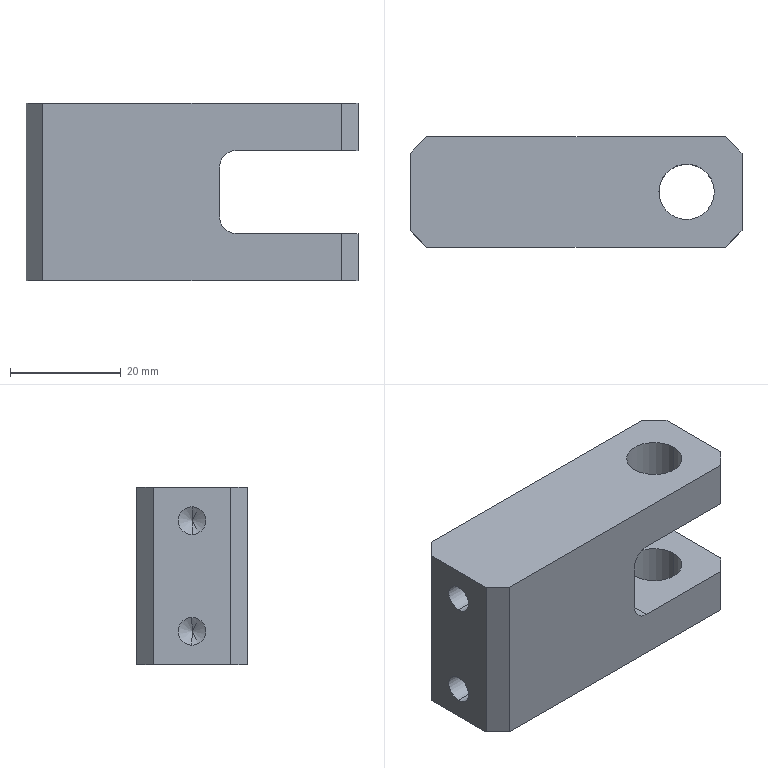Part | SolidWorks | features ICE 2, Chamfer 1, Extrusion 1, Fillet 1, HoleWzd 1 | 1 solid | 30 faces | box 60 x 20 x 32 mm | volume 28592 mm3 | plane 16 | cylinder 10 | cone 4 | commonest cylinder face diameters 5 x4 10 x4 6 x2
STEP:
#1=CARTESIAN_POINT('',(-15.,10.,-12.5));
#2=VERTEX_POINT('',#1);
#3=CARTESIAN_POINT('',(-15.,10.,-7.5));
#4=VERTEX_POINT('',#3);
#5=CARTESIAN_POINT('',(-15.,10.,-10.));
#6=DIRECTION('',(-1.,0.,0.));
#7=DIRECTION('',(0.,0.,1.));
#8=AXIS2_PLACEMENT_3D('',#5,#6,#7);
#9=CIRCLE('',#8,2.5);
#10=EDGE_CURVE('',#2,#4,#9,.T.);
#11=ORIENTED_EDGE('',*,*,#10,.F.);
#12=CARTESIAN_POINT('',(-30.,10.,-12.5));
#13=VERTEX_POINT('',#12);
#14=CARTESIAN_POINT('',(-30.,10.,-12.5));
#15=DIRECTION('',(-1.,0.,0.));
#16=VECTOR('',#15,1000.);
#17=LINE('',#14,#16);
#18=EDGE_CURVE('',#2,#13,#17,.T.);
#19=ORIENTED_EDGE('',*,*,#18,.T.);
#20=CARTESIAN_POINT('',(-30.,10.,-7.5));
#21=VERTEX_POINT('',#20);
#22=CARTESIAN_POINT('',(-30.,10.,-10.));
#23=DIRECTION('',(-1.,0.,0.));
#24=DIRECTION('',(0.,0.,1.));
#25=AXIS2_PLACEMENT_3D('',#22,#23,#24);
#26=CIRCLE('',#25,2.5);
#27=EDGE_CURVE('',#13,#21,#26,.T.);
#28=ORIENTED_EDGE('',*,*,#27,.T.);
#29=CARTESIAN_POINT('',(-30.,10.,-7.5));
#30=DIRECTION('',(-1.,0.,0.));
#31=VECTOR('',#30,1000.);
#32=LINE('',#29,#31);
#33=EDGE_CURVE('',#4,#21,#32,.T.);
#34=ORIENTED_EDGE('',*,*,#33,.F.);
#35=EDGE_LOOP('',(#11,#19,#28,#34));
#36=FACE_OUTER_BOUND('',#35,.T.);
#37=CARTESIAN_POINT('',(-30.,10.,-10.));
#38=DIRECTION('',(-1.,0.,0.));
#39=DIRECTION('',(0.,0.,1.));
#40=AXIS2_PLACEMENT_3D('',#37,#38,#39);
#41=CYLINDRICAL_SURFACE('',#40,2.5);
#42=ADVANCED_FACE('',(#36),#41,.F.);
#43=CARTESIAN_POINT('',(-13.498,10.,-10.));
#44=VERTEX_POINT('',#43);
#45=CARTESIAN_POINT('',(-15.,10.,-7.5));
#46=DIRECTION('',(-0.515,0.,0.8572));
#47=VECTOR('',#46,1000.);
#48=LINE('',#45,#47);
#49=EDGE_CURVE('',#44,#4,#48,.T.);
#50=ORIENTED_EDGE('',*,*,#49,.F.);
#51=CARTESIAN_POINT('',(-15.,10.,-12.5));
#52=DIRECTION('',(-0.515,0.,-0.8572));
#53=VECTOR('',#52,1000.);
#54=LINE('',#51,#53);
#55=EDGE_CURVE('',#44,#2,#54,.T.);
#56=ORIENTED_EDGE('',*,*,#55,.T.);
#57=ORIENTED_EDGE('',*,*,#10,.T.);
#58=EDGE_LOOP('',(#50,#56,#57));
#59=FACE_OUTER_BOUND('',#58,.T.);
#60=CARTESIAN_POINT('',(-15.,10.,-10.));
#61=DIRECTION('',(-1.,0.,0.));
#62=DIRECTION('',(0.,0.,1.));
#63=AXIS2_PLACEMENT_3D('',#60,#61,#62);
#64=CONICAL_SURFACE('',#63,2.5,1.03);
#65=ADVANCED_FACE('',(#59),#64,.F.);
#66=CARTESIAN_POINT('',(-15.,10.,7.5));
#67=VERTEX_POINT('',#66);
#68=CARTESIAN_POINT('',(-15.,10.,12.5));
#69=VERTEX_POINT('',#68);
#70=CARTESIAN_POINT('',(-15.,10.,10.));
#71=DIRECTION('',(-1.,0.,0.));
#72=DIRECTION('',(0.,0.,1.));
#73=AXIS2_PLACEMENT_3D('',#70,#71,#72);
#74=CIRCLE('',#73,2.5);
#75=EDGE_CURVE('',#67,#69,#74,.T.);
#76=ORIENTED_EDGE('',*,*,#75,.F.);
#77=CARTESIAN_POINT('',(-30.,10.,7.5));
#78=VERTEX_POINT('',#77);
#79=CARTESIAN_POINT('',(-30.,10.,7.5));
#80=DIRECTION('',(-1.,0.,0.));
#81=VECTOR('',#80,1000.);
#82=LINE('',#79,#81);
#83=EDGE_CURVE('',#67,#78,#82,.T.);
#84=ORIENTED_EDGE('',*,*,#83,.T.);
#85=CARTESIAN_POINT('',(-30.,10.,12.5));
#86=VERTEX_POINT('',#85);
#87=CARTESIAN_POINT('',(-30.,10.,10.));
#88=DIRECTION('',(-1.,0.,0.));
#89=DIRECTION('',(0.,0.,1.));
#90=AXIS2_PLACEMENT_3D('',#87,#88,#89);
#91=CIRCLE('',#90,2.5);
#92=EDGE_CURVE('',#78,#86,#91,.T.);
#93=ORIENTED_EDGE('',*,*,#92,.T.);
#94=CARTESIAN_POINT('',(-30.,10.,12.5));
#95=DIRECTION('',(-1.,0.,0.));
#96=VECTOR('',#95,1000.);
#97=LINE('',#94,#96);
#98=EDGE_CURVE('',#69,#86,#97,.T.);
#99=ORIENTED_EDGE('',*,*,#98,.F.);
#100=EDGE_LOOP('',(#76,#84,#93,#99));
#101=FACE_OUTER_BOUND('',#100,.T.);
#102=CARTESIAN_POINT('',(-30.,10.,10.));
#103=DIRECTION('',(-1.,0.,0.));
#104=DIRECTION('',(0.,0.,1.));
#105=AXIS2_PLACEMENT_3D('',#102,#103,#104);
#106=CYLINDRICAL_SURFACE('',#105,2.5);
#107=ADVANCED_FACE('',(#101),#106,.F.);
#108=CARTESIAN_POINT('',(-13.498,10.,10.));
#109=VERTEX_POINT('',#108);
#110=CARTESIAN_POINT('',(-15.,10.,12.5));
#111=DIRECTION('',(-0.515,0.,0.8572));
#112=VECTOR('',#111,1000.);
#113=LINE('',#110,#112);
#114=EDGE_CURVE('',#109,#69,#113,.T.);
#115=ORIENTED_EDGE('',*,*,#114,.F.);
#116=CARTESIAN_POINT('',(-15.,10.,7.5));
#117=DIRECTION('',(-0.515,0.,-0.8572));
#118=VECTOR('',#117,1000.);
#119=LINE('',#116,#118);
#120=EDGE_CURVE('',#109,#67,#119,.T.);
#121=ORIENTED_EDGE('',*,*,#120,.T.);
#122=ORIENTED_EDGE('',*,*,#75,.T.);
#123=EDGE_LOOP('',(#115,#121,#122));
#124=FACE_OUTER_BOUND('',#123,.T.);
#125=CARTESIAN_POINT('',(-15.,10.,10.));
#126=DIRECTION('',(-1.,0.,0.));
#127=DIRECTION('',(0.,0.,1.));
#128=AXIS2_PLACEMENT_3D('',#125,#126,#127);
#129=CONICAL_SURFACE('',#128,2.5,1.03);
#130=ADVANCED_FACE('',(#124),#129,.F.);
#131=CARTESIAN_POINT('',(25.,10.,7.5));
#132=VERTEX_POINT('',#131);
#133=CARTESIAN_POINT('',(15.,10.,7.5));
#134=VERTEX_POINT('',#133);
#135=CARTESIAN_POINT('',(20.,10.,7.5));
#136=DIRECTION('',(0.,0.,-1.));
#137=DIRECTION('',(1.,0.,0.));
#138=AXIS2_PLACEMENT_3D('',#135,#136,#137);
#139=CIRCLE('',#138,5.);
#140=EDGE_CURVE('',#132,#134,#139,.T.);
#141=ORIENTED_EDGE('',*,*,#140,.T.);
#142=CARTESIAN_POINT('',(15.,10.,16.));
#143=VERTEX_POINT('',#142);
#144=CARTESIAN_POINT('',(15.,10.,-26.));
#145=DIRECTION('',(0.,0.,1.));
#146=VECTOR('',#145,1000.);
#147=LINE('',#144,#146);
#148=EDGE_CURVE('',#134,#143,#147,.T.);
#149=ORIENTED_EDGE('',*,*,#148,.T.);
#150=CARTESIAN_POINT('',(25.,10.,16.));
#151=VERTEX_POINT('',#150);
#152=CARTESIAN_POINT('',(20.,10.,16.));
#153=DIRECTION('',(0.,0.,1.));
#154=DIRECTION('',(1.,0.,0.));
#155=AXIS2_PLACEMENT_3D('',#152,#153,#154);
#156=CIRCLE('',#155,5.);
#157=EDGE_CURVE('',#143,#151,#156,.T.);
#158=ORIENTED_EDGE('',*,*,#157,.T.);
#159=CARTESIAN_POINT('',(25.,10.,-26.));
#160=DIRECTION('',(0.,0.,1.));
#161=VECTOR('',#160,1000.);
#162=LINE('',#159,#161);
#163=EDGE_CURVE('',#132,#151,#162,.T.);
#164=ORIENTED_EDGE('',*,*,#163,.F.);
#165=EDGE_LOOP('',(#141,#149,#158,#164));
#166=FACE_OUTER_BOUND('',#165,.T.);
#167=CARTESIAN_POINT('',(20.,10.,-26.));
#168=DIRECTION('',(0.,0.,1.));
#169=DIRECTION('',(1.,0.,0.));
#170=AXIS2_PLACEMENT_3D('',#167,#168,#169);
#171=CYLINDRICAL_SURFACE('',#170,5.);
#172=ADVANCED_FACE('',(#166),#171,.F.);
#173=CARTESIAN_POINT('',(25.,10.,-16.));
#174=VERTEX_POINT('',#173);
#175=CARTESIAN_POINT('',(15.,10.,-16.));
#176=VERTEX_POINT('',#175);
#177=CARTESIAN_POINT('',(20.,10.,-16.));
#178=DIRECTION('',(0.,0.,-1.));
#179=DIRECTION('',(-1.,0.,0.));
#180=AXIS2_PLACEMENT_3D('',#177,#178,#179);
#181=CIRCLE('',#180,5.);
#182=EDGE_CURVE('',#174,#176,#181,.T.);
#183=ORIENTED_EDGE('',*,*,#182,.T.);
#184=CARTESIAN_POINT('',(15.,10.,-7.5));
#185=VERTEX_POINT('',#184);
#186=CARTESIAN_POINT('',(15.,10.,-26.));
#187=DIRECTION('',(0.,0.,1.));
#188=VECTOR('',#187,1000.);
#189=LINE('',#186,#188);
#190=EDGE_CURVE('',#176,#185,#189,.T.);
#191=ORIENTED_EDGE('',*,*,#190,.T.);
#192=CARTESIAN_POINT('',(25.,10.,-7.5));
#193=VERTEX_POINT('',#192);
#194=CARTESIAN_POINT('',(20.,10.,-7.5));
#195=DIRECTION('',(0.,0.,1.));
#196=DIRECTION('',(-1.,0.,0.));
#197=AXIS2_PLACEMENT_3D('',#194,#195,#196);
#198=CIRCLE('',#197,5.);
#199=EDGE_CURVE('',#185,#193,#198,.T.);
#200=ORIENTED_EDGE('',*,*,#199,.T.);
#201=CARTESIAN_POINT('',(25.,10.,-26.));
#202=DIRECTION('',(0.,0.,1.));
#203=VECTOR('',#202,1000.);
#204=LINE('',#201,#203);
#205=EDGE_CURVE('',#174,#193,#204,.T.);
#206=ORIENTED_EDGE('',*,*,#205,.F.);
#207=EDGE_LOOP('',(#183,#191,#200,#206));
#208=FACE_OUTER_BOUND('',#207,.T.);
#209=CARTESIAN_POINT('',(20.,10.,-26.));
#210=DIRECTION('',(0.,0.,1.));
#211=DIRECTION('',(1.,0.,0.));
#212=AXIS2_PLACEMENT_3D('',#209,#210,#211);
#213=CYLINDRICAL_SURFACE('',#212,5.);
#214=ADVANCED_FACE('',(#208),#213,.F.);
#215=CARTESIAN_POINT('',(30.,3.,-7.5));
#216=VERTEX_POINT('',#215);
#217=CARTESIAN_POINT('',(30.,17.,-7.5));
#218=VERTEX_POINT('',#217);
#219=CARTESIAN_POINT('',(30.,25.,-7.5));
#220=DIRECTION('',(0.,1.,0.));
#221=VECTOR('',#220,1000.);
#222=LINE('',#219,#221);
#223=EDGE_CURVE('',#216,#218,#222,.T.);
#224=ORIENTED_EDGE('',*,*,#223,.F.);
#225=CARTESIAN_POINT('',(30.,3.,-16.));
#226=VERTEX_POINT('',#225);
#227=CARTESIAN_POINT('',(30.,3.,-16.));
#228=DIRECTION('',(0.,0.,-1.));
#229=VECTOR('',#228,1000.);
#230=LINE('',#227,#229);
#231=EDGE_CURVE('',#216,#226,#230,.T.);
#232=ORIENTED_EDGE('',*,*,#231,.T.);
#233=CARTESIAN_POINT('',(30.,17.,-16.));
#234=VERTEX_POINT('',#233);
#235=CARTESIAN_POINT('',(30.,20.,-16.));
#236=DIRECTION('',(0.,-1.,0.));
#237=VECTOR('',#236,1000.);
#238=LINE('',#235,#237);
#239=EDGE_CURVE('',#234,#226,#238,.T.);
#240=ORIENTED_EDGE('',*,*,#239,.F.);
#241=CARTESIAN_POINT('',(30.,17.,-16.));
#242=DIRECTION('',(0.,0.,1.));
#243=VECTOR('',#242,1000.);
#244=LINE('',#241,#243);
#245=EDGE_CURVE('',#234,#218,#244,.T.);
#246=ORIENTED_EDGE('',*,*,#245,.T.);
#247=EDGE_LOOP('',(#224,#232,#240,#246));
#248=FACE_OUTER_BOUND('',#247,.T.);
#249=CARTESIAN_POINT('',(30.,20.,-16.));
#250=DIRECTION('',(1.,0.,0.));
#251=DIRECTION('',(0.,0.,-1.));
#252=AXIS2_PLACEMENT_3D('',#249,#250,#251);
#253=PLANE('',#252);
#254=ADVANCED_FACE('',(#248),#253,.T.);
#255=ORIENTED_EDGE('',*,*,#190,.F.);
#256=CARTESIAN_POINT('',(20.,10.,-16.));
#257=DIRECTION('',(0.,0.,-1.));
#258=DIRECTION('',(-1.,0.,0.));
#259=AXIS2_PLACEMENT_3D('',#256,#257,#258);
#260=CIRCLE('',#259,5.);
#261=EDGE_CURVE('',#176,#174,#260,.T.);
#262=ORIENTED_EDGE('',*,*,#261,.T.);
#263=ORIENTED_EDGE('',*,*,#205,.T.);
#264=CARTESIAN_POINT('',(20.,10.,-7.5));
#265=DIRECTION('',(0.,0.,1.));
#266=DIRECTION('',(-1.,0.,0.));
#267=AXIS2_PLACEMENT_3D('',#264,#265,#266);
#268=CIRCLE('',#267,5.);
#269=EDGE_CURVE('',#193,#185,#268,.T.);
#270=ORIENTED_EDGE('',*,*,#269,.T.);
#271=EDGE_LOOP('',(#255,#262,#263,#270));
#272=FACE_OUTER_BOUND('',#271,.T.);
#273=CARTESIAN_POINT('',(20.,10.,-26.));
#274=DIRECTION('',(0.,0.,1.));
#275=DIRECTION('',(1.,0.,0.));
#276=AXIS2_PLACEMENT_3D('',#273,#274,#275);
#277=CYLINDRICAL_SURFACE('',#276,5.);
#278=ADVANCED_FACE('',(#272),#277,.F.);
#279=CARTESIAN_POINT('',(27.,0.,-7.5));
#280=VERTEX_POINT('',#279);
#281=CARTESIAN_POINT('',(27.,0.,-7.5));
#282=DIRECTION('',(0.7071,0.7071,0.));
#283=VECTOR('',#282,1000.);
#284=LINE('',#281,#283);
#285=EDGE_CURVE('',#280,#216,#284,.T.);
#286=ORIENTED_EDGE('',*,*,#285,.F.);
#287=CARTESIAN_POINT('',(27.,0.,-16.));
#288=VERTEX_POINT('',#287);
#289=CARTESIAN_POINT('',(27.,0.,16.));
#290=DIRECTION('',(0.,0.,1.));
#291=VECTOR('',#290,1000.);
#292=LINE('',#289,#291);
#293=EDGE_CURVE('',#288,#280,#292,.T.);
#294=ORIENTED_EDGE('',*,*,#293,.F.);
#295=CARTESIAN_POINT('',(8.5,-18.5,-16.));
#296=DIRECTION('',(-0.7071,-0.7071,0.));
#297=VECTOR('',#296,1000.);
#298=LINE('',#295,#297);
#299=EDGE_CURVE('',#226,#288,#298,.T.);
#300=ORIENTED_EDGE('',*,*,#299,.F.);
#301=ORIENTED_EDGE('',*,*,#231,.F.);
#302=EDGE_LOOP('',(#286,#294,#300,#301));
#303=FACE_OUTER_BOUND('',#302,.T.);
#304=CARTESIAN_POINT('',(27.,0.,0.));
#305=DIRECTION('',(0.7071,-0.7071,0.));
#306=DIRECTION('',(0.,0.,-1.));
#307=AXIS2_PLACEMENT_3D('',#304,#305,#306);
#308=PLANE('',#307);
#309=ADVANCED_FACE('',(#303),#308,.T.);
#310=CARTESIAN_POINT('',(27.,20.,-7.5));
#311=VERTEX_POINT('',#310);
#312=CARTESIAN_POINT('',(30.,17.,-7.5));
#313=DIRECTION('',(-0.7071,0.7071,0.));
#314=VECTOR('',#313,1000.);
#315=LINE('',#312,#314);
#316=EDGE_CURVE('',#218,#311,#315,.T.);
#317=ORIENTED_EDGE('',*,*,#316,.F.);
#318=ORIENTED_EDGE('',*,*,#245,.F.);
#319=CARTESIAN_POINT('',(27.,20.,-16.));
#320=VERTEX_POINT('',#319);
#321=CARTESIAN_POINT('',(-1.5,48.5,-16.));
#322=DIRECTION('',(0.7071,-0.7071,0.));
#323=VECTOR('',#322,1000.);
#324=LINE('',#321,#323);
#325=EDGE_CURVE('',#320,#234,#324,.T.);
#326=ORIENTED_EDGE('',*,*,#325,.F.);
#327=CARTESIAN_POINT('',(27.,20.,0.));
#328=DIRECTION('',(0.,0.,-1.));
#329=VECTOR('',#328,1000.);
#330=LINE('',#327,#329);
#331=EDGE_CURVE('',#311,#320,#330,.T.);
#332=ORIENTED_EDGE('',*,*,#331,.F.);
#333=EDGE_LOOP('',(#317,#318,#326,#332));
#334=FACE_OUTER_BOUND('',#333,.T.);
#335=CARTESIAN_POINT('',(30.,17.,-16.));
#336=DIRECTION('',(-0.7071,-0.7071,0.));
#337=DIRECTION('',(0.,0.,1.));
#338=AXIS2_PLACEMENT_3D('',#335,#336,#337);
#339=PLANE('',#338);
#340=ADVANCED_FACE('',(#334),#339,.F.);
#341=CARTESIAN_POINT('',(-30.,10.,-10.));
#342=DIRECTION('',(-1.,0.,0.));
#343=DIRECTION('',(0.,0.,1.));
#344=AXIS2_PLACEMENT_3D('',#341,#342,#343);
#345=CIRCLE('',#344,2.5);
#346=EDGE_CURVE('',#21,#13,#345,.T.);
#347=ORIENTED_EDGE('',*,*,#346,.F.);
#348=ORIENTED_EDGE('',*,*,#27,.F.);
#349=EDGE_LOOP('',(#347,#348));
#350=FACE_BOUND('',#349,.T.);
#351=CARTESIAN_POINT('',(-30.,10.,10.));
#352=DIRECTION('',(-1.,0.,0.));
#353=DIRECTION('',(0.,0.,1.));
#354=AXIS2_PLACEMENT_3D('',#351,#352,#353);
#355=CIRCLE('',#354,2.5);
#356=EDGE_CURVE('',#86,#78,#355,.T.);
#357=ORIENTED_EDGE('',*,*,#356,.F.);
#358=ORIENTED_EDGE('',*,*,#92,.F.);
#359=EDGE_LOOP('',(#357,#358));
#360=FACE_BOUND('',#359,.T.);
#361=CARTESIAN_POINT('',(-30.,17.,-16.));
#362=VERTEX_POINT('',#361);
#363=CARTESIAN_POINT('',(-30.,3.,-16.));
#364=VERTEX_POINT('',#363);
#365=CARTESIAN_POINT('',(-30.,20.,-16.));
#366=DIRECTION('',(0.,-1.,0.));
#367=VECTOR('',#366,1000.);
#368=LINE('',#365,#367);
#369=EDGE_CURVE('',#362,#364,#368,.T.);
#370=ORIENTED_EDGE('',*,*,#369,.T.);
#371=CARTESIAN_POINT('',(-30.,3.,16.));
#372=VERTEX_POINT('',#371);
#373=CARTESIAN_POINT('',(-30.,3.,-16.));
#374=DIRECTION('',(0.,0.,1.));
#375=VECTOR('',#374,1000.);
#376=LINE('',#373,#375);
#377=EDGE_CURVE('',#364,#372,#376,.T.);
#378=ORIENTED_EDGE('',*,*,#377,.T.);
#379=CARTESIAN_POINT('',(-30.,17.,16.));
#380=VERTEX_POINT('',#379);
#381=CARTESIAN_POINT('',(-30.,20.,16.));
#382=DIRECTION('',(0.,-1.,0.));
#383=VECTOR('',#382,1000.);
#384=LINE('',#381,#383);
#385=EDGE_CURVE('',#380,#372,#384,.T.);
#386=ORIENTED_EDGE('',*,*,#385,.F.);
#387=CARTESIAN_POINT('',(-30.,17.,-16.));
#388=DIRECTION('',(0.,0.,-1.));
#389=VECTOR('',#388,1000.);
#390=LINE('',#387,#389);
#391=EDGE_CURVE('',#380,#362,#390,.T.);
#392=ORIENTED_EDGE('',*,*,#391,.T.);
#393=EDGE_LOOP('',(#370,#378,#386,#392));
#394=FACE_OUTER_BOUND('',#393,.T.);
#395=CARTESIAN_POINT('',(-30.,20.,-16.));
#396=DIRECTION('',(1.,0.,0.));
#397=DIRECTION('',(0.,0.,-1.));
#398=AXIS2_PLACEMENT_3D('',#395,#396,#397);
#399=PLANE('',#398);
#400=ADVANCED_FACE('',(#350,#360,#394),#399,.F.);
#401=CARTESIAN_POINT('',(20.,10.,16.));
#402=DIRECTION('',(0.,0.,1.));
#403=DIRECTION('',(1.,0.,0.));
#404=AXIS2_PLACEMENT_3D('',#401,#402,#403);
#405=CIRCLE('',#404,5.);
#406=EDGE_CURVE('',#151,#143,#405,.T.);
#407=ORIENTED_EDGE('',*,*,#406,.F.);
#408=ORIENTED_EDGE('',*,*,#157,.F.);
#409=EDGE_LOOP('',(#407,#408));
#410=FACE_BOUND('',#409,.T.);
#411=ORIENTED_EDGE('',*,*,#385,.T.);
#412=CARTESIAN_POINT('',(-27.,0.,16.));
#413=VERTEX_POINT('',#412);
#414=CARTESIAN_POINT('',(-30.,3.,16.));
#415=DIRECTION('',(0.7071,-0.7071,0.));
#416=VECTOR('',#415,1000.);
#417=LINE('',#414,#416);
#418=EDGE_CURVE('',#372,#413,#417,.T.);
#419=ORIENTED_EDGE('',*,*,#418,.T.);
#420=CARTESIAN_POINT('',(27.,0.,16.));
#421=VERTEX_POINT('',#420);
#422=CARTESIAN_POINT('',(-30.,0.,16.));
#423=DIRECTION('',(1.,0.,0.));
#424=VECTOR('',#423,1000.);
#425=LINE('',#422,#424);
#426=EDGE_CURVE('',#413,#421,#425,.T.);
#427=ORIENTED_EDGE('',*,*,#426,.T.);
#428=CARTESIAN_POINT('',(30.,3.,16.));
#429=VERTEX_POINT('',#428);
#430=CARTESIAN_POINT('',(27.,0.,16.));
#431=DIRECTION('',(0.7071,0.7071,0.));
#432=VECTOR('',#431,1000.);
#433=LINE('',#430,#432);
#434=EDGE_CURVE('',#421,#429,#433,.T.);
#435=ORIENTED_EDGE('',*,*,#434,.T.);
#436=CARTESIAN_POINT('',(30.,17.,16.));
#437=VERTEX_POINT('',#436);
#438=CARTESIAN_POINT('',(30.,20.,16.));
#439=DIRECTION('',(0.,-1.,0.));
#440=VECTOR('',#439,1000.);
#441=LINE('',#438,#440);
#442=EDGE_CURVE('',#437,#429,#441,.T.);
#443=ORIENTED_EDGE('',*,*,#442,.F.);
#444=CARTESIAN_POINT('',(27.,20.,16.));
#445=VERTEX_POINT('',#444);
#446=CARTESIAN_POINT('',(30.,17.,16.));
#447=DIRECTION('',(-0.7071,0.7071,0.));
#448=VECTOR('',#447,1000.);
#449=LINE('',#446,#448);
#450=EDGE_CURVE('',#437,#445,#449,.T.);
#451=ORIENTED_EDGE('',*,*,#450,.T.);
#452=CARTESIAN_POINT('',(-27.,20.,16.));
#453=VERTEX_POINT('',#452);
#454=CARTESIAN_POINT('',(-30.,20.,16.));
#455=DIRECTION('',(1.,0.,0.));
#456=VECTOR('',#455,1000.);
#457=LINE('',#454,#456);
#458=EDGE_CURVE('',#453,#445,#457,.T.);
#459=ORIENTED_EDGE('',*,*,#458,.F.);
#460=CARTESIAN_POINT('',(-27.,20.,16.));
#461=DIRECTION('',(-0.7071,-0.7071,0.));
#462=VECTOR('',#461,1000.);
#463=LINE('',#460,#462);
#464=EDGE_CURVE('',#453,#380,#463,.T.);
#465=ORIENTED_EDGE('',*,*,#464,.T.);
#466=EDGE_LOOP('',(#411,#419,#427,#435,#443,#451,#459,#465));
#467=FACE_OUTER_BOUND('',#466,.T.);
#468=CARTESIAN_POINT('',(-30.,20.,16.));
#469=DIRECTION('',(0.,0.,-1.));
#470=DIRECTION('',(-1.,0.,0.));
#471=AXIS2_PLACEMENT_3D('',#468,#469,#470);
#472=PLANE('',#471);
#473=ADVANCED_FACE('',(#410,#467),#472,.F.);
#474=CARTESIAN_POINT('',(30.,17.,7.5));
#475=VERTEX_POINT('',#474);
#476=CARTESIAN_POINT('',(30.,3.,7.5));
#477=VERTEX_POINT('',#476);
#478=CARTESIAN_POINT('',(30.,25.,7.5));
#479=DIRECTION('',(0.,-1.,0.));
#480=VECTOR('',#479,1000.);
#481=LINE('',#478,#480);
#482=EDGE_CURVE('',#475,#477,#481,.T.);
#483=ORIENTED_EDGE('',*,*,#482,.F.);
#484=CARTESIAN_POINT('',(30.,17.,-16.));
#485=DIRECTION('',(0.,0.,1.));
#486=VECTOR('',#485,1000.);
#487=LINE('',#484,#486);
#488=EDGE_CURVE('',#475,#437,#487,.T.);
#489=ORIENTED_EDGE('',*,*,#488,.T.);
#490=ORIENTED_EDGE('',*,*,#442,.T.);
#491=CARTESIAN_POINT('',(30.,3.,-16.));
#492=DIRECTION('',(0.,0.,-1.));
#493=VECTOR('',#492,1000.);
#494=LINE('',#491,#493);
#495=EDGE_CURVE('',#429,#477,#494,.T.);
#496=ORIENTED_EDGE('',*,*,#495,.T.);
#497=EDGE_LOOP('',(#483,#489,#490,#496));
#498=FACE_OUTER_BOUND('',#497,.T.);
#499=CARTESIAN_POINT('',(30.,20.,-16.));
#500=DIRECTION('',(1.,0.,0.));
#501=DIRECTION('',(0.,0.,-1.));
#502=AXIS2_PLACEMENT_3D('',#499,#500,#501);
#503=PLANE('',#502);
#504=ADVANCED_FACE('',(#498),#503,.T.);
#505=ORIENTED_EDGE('',*,*,#182,.F.);
#506=ORIENTED_EDGE('',*,*,#261,.F.);
#507=EDGE_LOOP('',(#505,#506));
#508=FACE_BOUND('',#507,.T.);
#509=CARTESIAN_POINT('',(-27.,0.,-16.));
#510=VERTEX_POINT('',#509);
#511=CARTESIAN_POINT('',(-30.,0.,-16.));
#512=DIRECTION('',(1.,0.,0.));
#513=VECTOR('',#512,1000.);
#514=LINE('',#511,#513);
#515=EDGE_CURVE('',#510,#288,#514,.T.);
#516=ORIENTED_EDGE('',*,*,#515,.F.);
#517=CARTESIAN_POINT('',(-38.5,11.5,-16.));
#518=DIRECTION('',(-0.7071,0.7071,0.));
#519=VECTOR('',#518,1000.);
#520=LINE('',#517,#519);
#521=EDGE_CURVE('',#510,#364,#520,.T.);
#522=ORIENTED_EDGE('',*,*,#521,.T.);
#523=ORIENTED_EDGE('',*,*,#369,.F.);
#524=CARTESIAN_POINT('',(-27.,20.,-16.));
#525=VERTEX_POINT('',#524);
#526=CARTESIAN_POINT('',(-28.5,18.5,-16.));
#527=DIRECTION('',(0.7071,0.7071,0.));
#528=VECTOR('',#527,1000.);
#529=LINE('',#526,#528);
#530=EDGE_CURVE('',#362,#525,#529,.T.);
#531=ORIENTED_EDGE('',*,*,#530,.T.);
#532=CARTESIAN_POINT('',(-30.,20.,-16.));
#533=DIRECTION('',(1.,0.,0.));
#534=VECTOR('',#533,1000.);
#535=LINE('',#532,#534);
#536=EDGE_CURVE('',#525,#320,#535,.T.);
#537=ORIENTED_EDGE('',*,*,#536,.T.);
#538=ORIENTED_EDGE('',*,*,#325,.T.);
#539=ORIENTED_EDGE('',*,*,#239,.T.);
#540=ORIENTED_EDGE('',*,*,#299,.T.);
#541=EDGE_LOOP('',(#516,#522,#523,#531,#537,#538,#539,#540));
#542=FACE_OUTER_BOUND('',#541,.T.);
#543=CARTESIAN_POINT('',(-30.,20.,-16.));
#544=DIRECTION('',(0.,0.,-1.));
#545=DIRECTION('',(-1.,0.,0.));
#546=AXIS2_PLACEMENT_3D('',#543,#544,#545);
#547=PLANE('',#546);
#548=ADVANCED_FACE('',(#508,#542),#547,.T.);
#549=CARTESIAN_POINT('',(8.,20.,-7.5));
#550=VERTEX_POINT('',#549);
#551=CARTESIAN_POINT('',(0.,20.,-7.5));
#552=DIRECTION('',(-1.,0.,0.));
#553=VECTOR('',#552,1000.);
#554=LINE('',#551,#553);
#555=EDGE_CURVE('',#311,#550,#554,.T.);
#556=ORIENTED_EDGE('',*,*,#555,.F.);
#557=ORIENTED_EDGE('',*,*,#331,.T.);
#558=ORIENTED_EDGE('',*,*,#536,.F.);
#559=CARTESIAN_POINT('',(-27.,20.,16.));
#560=DIRECTION('',(0.,0.,1.));
#561=VECTOR('',#560,1000.);
#562=LINE('',#559,#561);
#563=EDGE_CURVE('',#525,#453,#562,.T.);
#564=ORIENTED_EDGE('',*,*,#563,.T.);
#565=ORIENTED_EDGE('',*,*,#458,.T.);
#566=CARTESIAN_POINT('',(27.,20.,7.5));
#567=VERTEX_POINT('',#566);
#568=CARTESIAN_POINT('',(27.,20.,0.));
#569=DIRECTION('',(0.,0.,-1.));
#570=VECTOR('',#569,1000.);
#571=LINE('',#568,#570);
#572=EDGE_CURVE('',#445,#567,#571,.T.);
#573=ORIENTED_EDGE('',*,*,#572,.T.);
#574=CARTESIAN_POINT('',(8.,20.,7.5));
#575=VERTEX_POINT('',#574);
#576=CARTESIAN_POINT('',(0.,20.,7.5));
#577=DIRECTION('',(1.,0.,0.));
#578=VECTOR('',#577,1000.);
#579=LINE('',#576,#578);
#580=EDGE_CURVE('',#575,#567,#579,.T.);
#581=ORIENTED_EDGE('',*,*,#580,.F.);
#582=CARTESIAN_POINT('',(5.,20.,4.5));
#583=VERTEX_POINT('',#582);
#584=CARTESIAN_POINT('',(8.,20.,4.5));
#585=DIRECTION('',(0.,-1.,0.));
#586=DIRECTION('',(0.,0.,1.));
#587=AXIS2_PLACEMENT_3D('',#584,#585,#586);
#588=CIRCLE('',#587,3.);
#589=EDGE_CURVE('',#575,#583,#588,.T.);
#590=ORIENTED_EDGE('',*,*,#589,.T.);
#591=CARTESIAN_POINT('',(5.,20.,-4.5));
#592=VERTEX_POINT('',#591);
#593=CARTESIAN_POINT('',(5.,20.,0.));
#594=DIRECTION('',(0.,0.,-1.));
#595=VECTOR('',#594,1000.);
#596=LINE('',#593,#595);
#597=EDGE_CURVE('',#583,#592,#596,.T.);
#598=ORIENTED_EDGE('',*,*,#597,.T.);
#599=CARTESIAN_POINT('',(8.,20.,-4.5));
#600=DIRECTION('',(0.,-1.,0.));
#601=DIRECTION('',(0.,0.,1.));
#602=AXIS2_PLACEMENT_3D('',#599,#600,#601);
#603=CIRCLE('',#602,3.);
#604=EDGE_CURVE('',#592,#550,#603,.T.);
#605=ORIENTED_EDGE('',*,*,#604,.T.);
#606=EDGE_LOOP('',(#556,#557,#558,#564,#565,#573,#581,#590,#598,#605));
#607=FACE_OUTER_BOUND('',#606,.T.);
#608=CARTESIAN_POINT('',(0.,20.,0.));
#609=DIRECTION('',(0.,1.,0.));
#610=DIRECTION('',(0.,0.,1.));
#611=AXIS2_PLACEMENT_3D('',#608,#609,#610);
#612=PLANE('',#611);
#613=ADVANCED_FACE('',(#607),#612,.T.);
#614=ORIENTED_EDGE('',*,*,#293,.T.);
#615=CARTESIAN_POINT('',(8.,0.,-7.5));
#616=VERTEX_POINT('',#615);
#617=CARTESIAN_POINT('',(0.,0.,-7.5));
#618=DIRECTION('',(-1.,0.,0.));
#619=VECTOR('',#618,1000.);
#620=LINE('',#617,#619);
#621=EDGE_CURVE('',#280,#616,#620,.T.);
#622=ORIENTED_EDGE('',*,*,#621,.T.);
#623=CARTESIAN_POINT('',(5.,0.,-4.5));
#624=VERTEX_POINT('',#623);
#625=CARTESIAN_POINT('',(8.,0.,-4.5));
#626=DIRECTION('',(0.,1.,0.));
#627=DIRECTION('',(0.,0.,1.));
#628=AXIS2_PLACEMENT_3D('',#625,#626,#627);
#629=CIRCLE('',#628,3.);
#630=EDGE_CURVE('',#616,#624,#629,.T.);
#631=ORIENTED_EDGE('',*,*,#630,.T.);
#632=CARTESIAN_POINT('',(5.,0.,4.5));
#633=VERTEX_POINT('',#632);
#634=CARTESIAN_POINT('',(5.,0.,0.));
#635=DIRECTION('',(0.,0.,-1.));
#636=VECTOR('',#635,1000.);
#637=LINE('',#634,#636);
#638=EDGE_CURVE('',#633,#624,#637,.T.);
#639=ORIENTED_EDGE('',*,*,#638,.F.);
#640=CARTESIAN_POINT('',(8.,0.,7.5));
#641=VERTEX_POINT('',#640);
#642=CARTESIAN_POINT('',(8.,0.,4.5));
#643=DIRECTION('',(0.,1.,0.));
#644=DIRECTION('',(0.,0.,1.));
#645=AXIS2_PLACEMENT_3D('',#642,#643,#644);
#646=CIRCLE('',#645,3.);
#647=EDGE_CURVE('',#633,#641,#646,.T.);
#648=ORIENTED_EDGE('',*,*,#647,.T.);
#649=CARTESIAN_POINT('',(27.,0.,7.5));
#650=VERTEX_POINT('',#649);
#651=CARTESIAN_POINT('',(0.,0.,7.5));
#652=DIRECTION('',(1.,0.,0.));
#653=VECTOR('',#652,1000.);
#654=LINE('',#651,#653);
#655=EDGE_CURVE('',#641,#650,#654,.T.);
#656=ORIENTED_EDGE('',*,*,#655,.T.);
#657=CARTESIAN_POINT('',(27.,0.,16.));
#658=DIRECTION('',(0.,0.,1.));
#659=VECTOR('',#658,1000.);
#660=LINE('',#657,#659);
#661=EDGE_CURVE('',#650,#421,#660,.T.);
#662=ORIENTED_EDGE('',*,*,#661,.T.);
#663=ORIENTED_EDGE('',*,*,#426,.F.);
#664=CARTESIAN_POINT('',(-27.,0.,0.));
#665=DIRECTION('',(0.,0.,-1.));
#666=VECTOR('',#665,1000.);
#667=LINE('',#664,#666);
#668=EDGE_CURVE('',#413,#510,#667,.T.);
#669=ORIENTED_EDGE('',*,*,#668,.T.);
#670=ORIENTED_EDGE('',*,*,#515,.T.);
#671=EDGE_LOOP('',(#614,#622,#631,#639,#648,#656,#662,#663,#669,#670));
#672=FACE_OUTER_BOUND('',#671,.T.);
#673=CARTESIAN_POINT('',(0.,0.,0.));
#674=DIRECTION('',(0.,1.,0.));
#675=DIRECTION('',(0.,0.,1.));
#676=AXIS2_PLACEMENT_3D('',#673,#674,#675);
#677=PLANE('',#676);
#678=ADVANCED_FACE('',(#672),#677,.F.);
#679=ORIENTED_EDGE('',*,*,#148,.F.);
#680=CARTESIAN_POINT('',(20.,10.,7.5));
#681=DIRECTION('',(0.,0.,-1.));
#682=DIRECTION('',(1.,0.,0.));
#683=AXIS2_PLACEMENT_3D('',#680,#681,#682);
#684=CIRCLE('',#683,5.);
#685=EDGE_CURVE('',#134,#132,#684,.T.);
#686=ORIENTED_EDGE('',*,*,#685,.T.);
#687=ORIENTED_EDGE('',*,*,#163,.T.);
#688=ORIENTED_EDGE('',*,*,#406,.T.);
#689=EDGE_LOOP('',(#679,#686,#687,#688));
#690=FACE_OUTER_BOUND('',#689,.T.);
#691=CARTESIAN_POINT('',(20.,10.,-26.));
#692=DIRECTION('',(0.,0.,1.));
#693=DIRECTION('',(1.,0.,0.));
#694=AXIS2_PLACEMENT_3D('',#691,#692,#693);
#695=CYLINDRICAL_SURFACE('',#694,5.);
#696=ADVANCED_FACE('',(#690),#695,.F.);
#697=ORIENTED_EDGE('',*,*,#521,.F.);
#698=ORIENTED_EDGE('',*,*,#668,.F.);
#699=ORIENTED_EDGE('',*,*,#418,.F.);
#700=ORIENTED_EDGE('',*,*,#377,.F.);
#701=EDGE_LOOP('',(#697,#698,#699,#700));
#702=FACE_OUTER_BOUND('',#701,.T.);
#703=CARTESIAN_POINT('',(-30.,3.,-16.));
#704=DIRECTION('',(0.7071,0.7071,0.));
#705=DIRECTION('',(0.,0.,1.));
#706=AXIS2_PLACEMENT_3D('',#703,#704,#705);
#707=PLANE('',#706);
#708=ADVANCED_FACE('',(#702),#707,.F.);
#709=ORIENTED_EDGE('',*,*,#530,.F.);
#710=ORIENTED_EDGE('',*,*,#391,.F.);
#711=ORIENTED_EDGE('',*,*,#464,.F.);
#712=ORIENTED_EDGE('',*,*,#563,.F.);
#713=EDGE_LOOP('',(#709,#710,#711,#712));
#714=FACE_OUTER_BOUND('',#713,.T.);
#715=CARTESIAN_POINT('',(-27.,20.,0.));
#716=DIRECTION('',(-0.7071,0.7071,0.));
#717=DIRECTION('',(0.,0.,-1.));
#718=AXIS2_PLACEMENT_3D('',#715,#716,#717);
#719=PLANE('',#718);
#720=ADVANCED_FACE('',(#714),#719,.T.);
#721=CARTESIAN_POINT('',(27.,0.,7.5));
#722=DIRECTION('',(-0.7071,-0.7071,0.));
#723=VECTOR('',#722,1000.);
#724=LINE('',#721,#723);
#725=EDGE_CURVE('',#477,#650,#724,.T.);
#726=ORIENTED_EDGE('',*,*,#725,.F.);
#727=ORIENTED_EDGE('',*,*,#495,.F.);
#728=ORIENTED_EDGE('',*,*,#434,.F.);
#729=ORIENTED_EDGE('',*,*,#661,.F.);
#730=EDGE_LOOP('',(#726,#727,#728,#729));
#731=FACE_OUTER_BOUND('',#730,.T.);
#732=CARTESIAN_POINT('',(27.,0.,0.));
#733=DIRECTION('',(0.7071,-0.7071,0.));
#734=DIRECTION('',(0.,0.,-1.));
#735=AXIS2_PLACEMENT_3D('',#732,#733,#734);
#736=PLANE('',#735);
#737=ADVANCED_FACE('',(#731),#736,.T.);
#738=CARTESIAN_POINT('',(30.,17.,7.5));
#739=DIRECTION('',(0.7071,-0.7071,0.));
#740=VECTOR('',#739,1000.);
#741=LINE('',#738,#740);
#742=EDGE_CURVE('',#567,#475,#741,.T.);
#743=ORIENTED_EDGE('',*,*,#742,.F.);
#744=ORIENTED_EDGE('',*,*,#572,.F.);
#745=ORIENTED_EDGE('',*,*,#450,.F.);
#746=ORIENTED_EDGE('',*,*,#488,.F.);
#747=EDGE_LOOP('',(#743,#744,#745,#746));
#748=FACE_OUTER_BOUND('',#747,.T.);
#749=CARTESIAN_POINT('',(30.,17.,-16.));
#750=DIRECTION('',(-0.7071,-0.7071,0.));
#751=DIRECTION('',(0.,0.,1.));
#752=AXIS2_PLACEMENT_3D('',#749,#750,#751);
#753=PLANE('',#752);
#754=ADVANCED_FACE('',(#748),#753,.F.);
#755=ORIENTED_EDGE('',*,*,#120,.F.);
#756=ORIENTED_EDGE('',*,*,#114,.T.);
#757=CARTESIAN_POINT('',(-15.,10.,10.));
#758=DIRECTION('',(-1.,0.,0.));
#759=DIRECTION('',(0.,0.,1.));
#760=AXIS2_PLACEMENT_3D('',#757,#758,#759);
#761=CIRCLE('',#760,2.5);
#762=EDGE_CURVE('',#69,#67,#761,.T.);
#763=ORIENTED_EDGE('',*,*,#762,.T.);
#764=EDGE_LOOP('',(#755,#756,#763));
#765=FACE_OUTER_BOUND('',#764,.T.);
#766=CARTESIAN_POINT('',(-15.,10.,10.));
#767=DIRECTION('',(-1.,0.,0.));
#768=DIRECTION('',(0.,0.,1.));
#769=AXIS2_PLACEMENT_3D('',#766,#767,#768);
#770=CONICAL_SURFACE('',#769,2.5,1.03);
#771=ADVANCED_FACE('',(#765),#770,.F.);
#772=ORIENTED_EDGE('',*,*,#83,.F.);
#773=ORIENTED_EDGE('',*,*,#762,.F.);
#774=ORIENTED_EDGE('',*,*,#98,.T.);
#775=ORIENTED_EDGE('',*,*,#356,.T.);
#776=EDGE_LOOP('',(#772,#773,#774,#775));
#777=FACE_OUTER_BOUND('',#776,.T.);
#778=CARTESIAN_POINT('',(-30.,10.,10.));
#779=DIRECTION('',(-1.,0.,0.));
#780=DIRECTION('',(0.,0.,1.));
#781=AXIS2_PLACEMENT_3D('',#778,#779,#780);
#782=CYLINDRICAL_SURFACE('',#781,2.5);
#783=ADVANCED_FACE('',(#777),#782,.F.);
#784=ORIENTED_EDGE('',*,*,#55,.F.);
#785=ORIENTED_EDGE('',*,*,#49,.T.);
#786=CARTESIAN_POINT('',(-15.,10.,-10.));
#787=DIRECTION('',(-1.,0.,0.));
#788=DIRECTION('',(0.,0.,1.));
#789=AXIS2_PLACEMENT_3D('',#786,#787,#788);
#790=CIRCLE('',#789,2.5);
#791=EDGE_CURVE('',#4,#2,#790,.T.);
#792=ORIENTED_EDGE('',*,*,#791,.T.);
#793=EDGE_LOOP('',(#784,#785,#792));
#794=FACE_OUTER_BOUND('',#793,.T.);
#795=CARTESIAN_POINT('',(-15.,10.,-10.));
#796=DIRECTION('',(-1.,0.,0.));
#797=DIRECTION('',(0.,0.,1.));
#798=AXIS2_PLACEMENT_3D('',#795,#796,#797);
#799=CONICAL_SURFACE('',#798,2.5,1.03);
#800=ADVANCED_FACE('',(#794),#799,.F.);
#801=ORIENTED_EDGE('',*,*,#18,.F.);
#802=ORIENTED_EDGE('',*,*,#791,.F.);
#803=ORIENTED_EDGE('',*,*,#33,.T.);
#804=ORIENTED_EDGE('',*,*,#346,.T.);
#805=EDGE_LOOP('',(#801,#802,#803,#804));
#806=FACE_OUTER_BOUND('',#805,.T.);
#807=CARTESIAN_POINT('',(-30.,10.,-10.));
#808=DIRECTION('',(-1.,0.,0.));
#809=DIRECTION('',(0.,0.,1.));
#810=AXIS2_PLACEMENT_3D('',#807,#808,#809);
#811=CYLINDRICAL_SURFACE('',#810,2.5);
#812=ADVANCED_FACE('',(#806),#811,.F.);
#813=ORIENTED_EDGE('',*,*,#597,.F.);
#814=CARTESIAN_POINT('',(5.,0.,4.5));
#815=DIRECTION('',(0.,-1.,0.));
#816=VECTOR('',#815,1000.);
#817=LINE('',#814,#816);
#818=EDGE_CURVE('',#583,#633,#817,.T.);
#819=ORIENTED_EDGE('',*,*,#818,.T.);
#820=ORIENTED_EDGE('',*,*,#638,.T.);
#821=CARTESIAN_POINT('',(5.,0.,-4.5));
#822=DIRECTION('',(0.,1.,0.));
#823=VECTOR('',#822,1000.);
#824=LINE('',#821,#823);
#825=EDGE_CURVE('',#624,#592,#824,.T.);
#826=ORIENTED_EDGE('',*,*,#825,.T.);
#827=EDGE_LOOP('',(#813,#819,#820,#826));
#828=FACE_OUTER_BOUND('',#827,.T.);
#829=CARTESIAN_POINT('',(5.,0.,0.));
#830=DIRECTION('',(1.,0.,0.));
#831=DIRECTION('',(0.,0.,-1.));
#832=AXIS2_PLACEMENT_3D('',#829,#830,#831);
#833=PLANE('',#832);
#834=ADVANCED_FACE('',(#828),#833,.T.);
#835=ORIENTED_EDGE('',*,*,#555,.T.);
#836=CARTESIAN_POINT('',(8.,25.,-7.5));
#837=DIRECTION('',(0.,-1.,0.));
#838=VECTOR('',#837,1000.);
#839=LINE('',#836,#838);
#840=EDGE_CURVE('',#550,#616,#839,.T.);
#841=ORIENTED_EDGE('',*,*,#840,.T.);
#842=ORIENTED_EDGE('',*,*,#621,.F.);
#843=ORIENTED_EDGE('',*,*,#285,.T.);
#844=ORIENTED_EDGE('',*,*,#223,.T.);
#845=ORIENTED_EDGE('',*,*,#316,.T.);
#846=EDGE_LOOP('',(#835,#841,#842,#843,#844,#845));
#847=FACE_OUTER_BOUND('',#846,.T.);
#848=ORIENTED_EDGE('',*,*,#269,.F.);
#849=ORIENTED_EDGE('',*,*,#199,.F.);
#850=EDGE_LOOP('',(#848,#849));
#851=FACE_BOUND('',#850,.T.);
#852=CARTESIAN_POINT('',(5.,25.,-7.5));
#853=DIRECTION('',(0.,0.,-1.));
#854=DIRECTION('',(-1.,0.,0.));
#855=AXIS2_PLACEMENT_3D('',#852,#853,#854);
#856=PLANE('',#855);
#857=ADVANCED_FACE('',(#847,#851),#856,.F.);
#858=ORIENTED_EDGE('',*,*,#655,.F.);
#859=CARTESIAN_POINT('',(8.,25.,7.5));
#860=DIRECTION('',(0.,1.,0.));
#861=VECTOR('',#860,1000.);
#862=LINE('',#859,#861);
#863=EDGE_CURVE('',#641,#575,#862,.T.);
#864=ORIENTED_EDGE('',*,*,#863,.T.);
#865=ORIENTED_EDGE('',*,*,#580,.T.);
#866=ORIENTED_EDGE('',*,*,#742,.T.);
#867=ORIENTED_EDGE('',*,*,#482,.T.);
#868=ORIENTED_EDGE('',*,*,#725,.T.);
#869=EDGE_LOOP('',(#858,#864,#865,#866,#867,#868));
#870=FACE_OUTER_BOUND('',#869,.T.);
#871=ORIENTED_EDGE('',*,*,#140,.F.);
#872=ORIENTED_EDGE('',*,*,#685,.F.);
#873=EDGE_LOOP('',(#871,#872));
#874=FACE_BOUND('',#873,.T.);
#875=CARTESIAN_POINT('',(5.,25.,7.5));
#876=DIRECTION('',(0.,0.,1.));
#877=DIRECTION('',(1.,0.,0.));
#878=AXIS2_PLACEMENT_3D('',#875,#876,#877);
#879=PLANE('',#878);
#880=ADVANCED_FACE('',(#870,#874),#879,.F.);
#881=ORIENTED_EDGE('',*,*,#589,.F.);
#882=ORIENTED_EDGE('',*,*,#863,.F.);
#883=ORIENTED_EDGE('',*,*,#647,.F.);
#884=ORIENTED_EDGE('',*,*,#818,.F.);
#885=EDGE_LOOP('',(#881,#882,#883,#884));
#886=FACE_OUTER_BOUND('',#885,.T.);
#887=CARTESIAN_POINT('',(8.,0.,4.5));
#888=DIRECTION('',(0.,-1.,0.));
#889=DIRECTION('',(0.,0.,-1.));
#890=AXIS2_PLACEMENT_3D('',#887,#888,#889);
#891=CYLINDRICAL_SURFACE('',#890,3.);
#892=ADVANCED_FACE('',(#886),#891,.F.);
#893=ORIENTED_EDGE('',*,*,#630,.F.);
#894=ORIENTED_EDGE('',*,*,#840,.F.);
#895=ORIENTED_EDGE('',*,*,#604,.F.);
#896=ORIENTED_EDGE('',*,*,#825,.F.);
#897=EDGE_LOOP('',(#893,#894,#895,#896));
#898=FACE_OUTER_BOUND('',#897,.T.);
#899=CARTESIAN_POINT('',(8.,0.,-4.5));
#900=DIRECTION('',(0.,1.,0.));
#901=DIRECTION('',(0.,0.,1.));
#902=AXIS2_PLACEMENT_3D('',#899,#900,#901);
#903=CYLINDRICAL_SURFACE('',#902,3.);
#904=ADVANCED_FACE('',(#898),#903,.F.);
#905=CLOSED_SHELL('',(#42,#65,#107,#130,#172,#214,#254,#278,#309,#340,#400,#473,#504,#548,#613,#678,#696,#708,#720,#737,#754,#771,#783,#800,#812,#834,#857,#880,#892,#904));
#906=MANIFOLD_SOLID_BREP('',#905);
#907=CARTESIAN_POINT('',(0.,0.,0.));
#908=DIRECTION('',(0.,0.,1.));
#909=DIRECTION('',(1.,0.,0.));
#910=AXIS2_PLACEMENT_3D('',#907,#908,#909);
#911=(LENGTH_UNIT()NAMED_UNIT(*)SI_UNIT(.MILLI.,.METRE.));
#912=UNCERTAINTY_MEASURE_WITH_UNIT(LENGTH_MEASURE(0.00001),#911,'','');
#913=(NAMED_UNIT(*)PLANE_ANGLE_UNIT()SI_UNIT($,.RADIAN.));
#914=(NAMED_UNIT(*)SI_UNIT($,.STERADIAN.)SOLID_ANGLE_UNIT());
#915=(GEOMETRIC_REPRESENTATION_CONTEXT(3)GLOBAL_UNCERTAINTY_ASSIGNED_CONTEXT((#912))GLOBAL_UNIT_ASSIGNED_CONTEXT((#911,#913,#914))REPRESENTATION_CONTEXT('',''));
#916=ADVANCED_BREP_SHAPE_REPRESENTATION('',(#906,#910),#915);